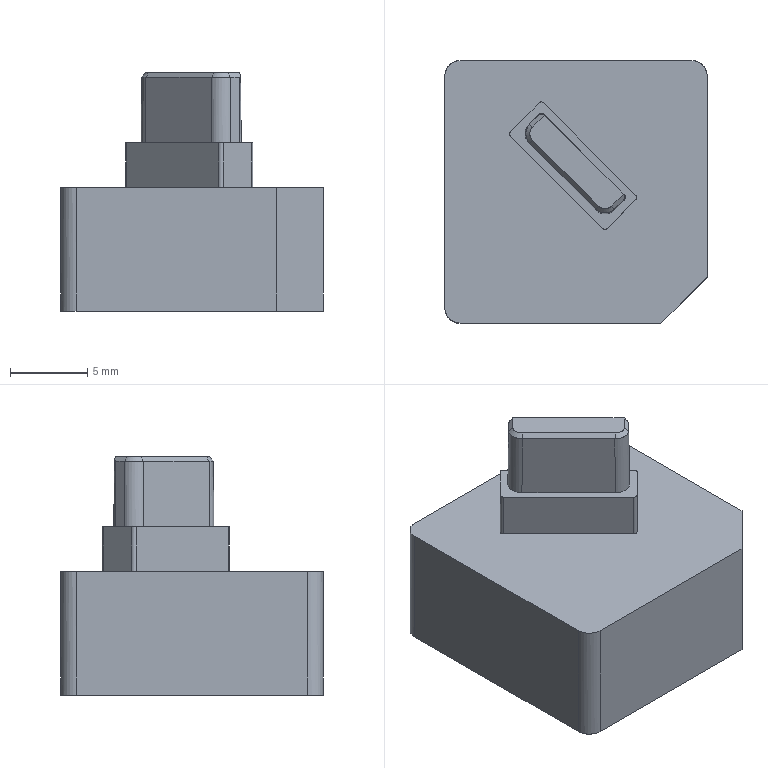NC program | PowerMill | posted with a generic post | part box 17 x 17 x 15.424 mm
Lines 38229 to 38437 of 38437:
N38326 M6
N38327 S15000 M03
N38328 G00 G90 X0.0 Y0.0
N38329 G43 Z10.304 H13
N38330
N38331 G05 P10000 R8
N38332 X-7.0355 Y-6.6806
N38333 Z-7.57
N38334 G01 Z-7.67
N38335 X-7.1957 Y-6.6713 F1000.0
N38336 X-7.3268 Y-6.6435
N38337 X-7.4288 Y-6.597
N38338 X-7.5016 Y-6.532
N38339 X-7.5453 Y-6.4484
N38340 X-7.5598 Y-6.3462
N38341 X-7.5453 Y-6.244
N38342 X-7.5016 Y-6.1604
N38343 X-7.4288 Y-6.0954
N38344 X-7.3268 Y-6.0489
N38345 X-7.1957 Y-6.0211
N38346 X-7.0355 Y-6.0118
N38347 X-6.8786 Y-6.021
N38348 X-6.7492 Y-6.0489
N38349 X-6.6473 Y-6.0953
N38350 X-6.573 Y-6.1602
N38351 X-6.5279 Y-6.2434
N38352 X-6.5128 Y-6.3462
N38353 X-6.5273 Y-6.4484
N38354 X-6.5709 Y-6.532
N38355 X-6.6435 Y-6.597
N38356 X-6.7451 Y-6.6435
N38357 X-6.8758 Y-6.6713
N38358 X-7.0355 Y-6.6806
N38359 G00 Z-4.4979
N38360 G01 X-6.5237 Y-5.0631 F10000.0
N38361 G00 Z-7.57
N38362 G01 Z-7.67 F600.0
N38363 X-7.5598 Y-5.0639 F1000.0
N38364 X-6.78 Y-5.6343
N38365 Y-4.9561
N38366 G00 Z-4.4979
N38367 G01 X-6.8918 Y-4.1114 F10000.0
N38368 G00 Z-7.57
N38369 G01 Z-7.67 F600.0
N38370 Y-4.5044 F1000.0
N38371 G00 Z-4.4979
N38372 G01 X-6.855 Y-2.7884 F10000.0
N38373 G00 Z-7.57
N38374 G01 Z-7.67 F600.0
N38375 X-6.7553 Y-2.8234 F1000.0
N38376 X-6.6717 Y-2.8732
N38377 X-6.6042 Y-2.9377
N38378 X-6.5534 Y-3.0172
N38379 X-6.523 Y-3.1089
N38380 X-6.5128 Y-3.2127
N38381 X-6.5233 Y-3.3314
N38382 X-6.5548 Y-3.4335
N38383 X-6.6073 Y-3.5192
N38384 X-6.6808 Y-3.5883
N38385 X-6.7753 Y-3.6409
N38386 X-6.9078 Y-3.6814
N38387 X-7.0504 Y-3.6948
N38388 X-7.2034 Y-3.6801
N38389 X-7.3311 Y-3.636
N38390 X-7.4335 Y-3.5625
N38391 X-7.5106 Y-3.4596
N38392 X-7.5575 Y-3.3409
N38393 X-7.5731 Y-3.2112
N38394 X-7.5646 Y-3.1148
N38395 X-7.5389 Y-3.0288
N38396 X-7.4962 Y-2.9533
N38397 X-7.4373 Y-2.89
N38398 X-7.3632 Y-2.8408
N38399 X-7.2739 Y-2.8056
N38400 G00 Z-4.4979
N38401 G01 X-7.1957 Y-2.3618 F10000.0
N38402 G00 Z-7.57
N38403 G01 Z-7.67 F600.0
N38404 X-7.3268 Y-2.334 F1000.0
N38405 X-7.4288 Y-2.2875
N38406 X-7.5016 Y-2.2225
N38407 X-7.5453 Y-2.1389
N38408 X-7.5598 Y-2.0367
N38409 X-7.5453 Y-1.9345
N38410 X-7.5016 Y-1.8509
N38411 X-7.4288 Y-1.7859
N38412 X-7.3268 Y-1.7394
N38413 X-7.1957 Y-1.7116
N38414 X-7.0355 Y-1.7023
N38415 X-6.8786 Y-1.7116
N38416 X-6.7492 Y-1.7394
N38417 X-6.6473 Y-1.7858
N38418 X-6.573 Y-1.8507
N38419 X-6.5279 Y-1.934
N38420 X-6.5128 Y-2.0367
N38421 X-6.5273 Y-2.1389
N38422 X-6.5709 Y-2.2225
N38423 X-6.6435 Y-2.2875
N38424 X-6.7451 Y-2.334
N38425 X-6.8758 Y-2.3618
N38426 X-7.0355 Y-2.3711
N38427 X-7.1957 Y-2.3618
N38428 G00 Z-4.4979
N38429 G01 X-7.4223 Y-0.9927 F10000.0
N38430 G00 Z-7.57
N38431 G01 Z-7.67 F600.0
N38432 X-7.5552 Y-0.7997 F1000.0
N38433 X-6.53
N38434 G00 Z-4.4979
N38435 G01 X-6.8918 Y0.1981 F10000.0
N38436 G00 Z-7.57
N38437 G01 Z-7.67 F600.0
N38438 Y-0.1949 F1000.0
N38439 G00 Z-4.4979
N38440 G01 X-6.5237 Y1.1225 F10000.0
N38441 G00 Z-7.57
N38442 G01 Z-7.67 F600.0
N38443 X-7.5598 Y1.1218 F1000.0
N38444 X-6.78 Y0.5514
N38445 Y1.2296
N38446 G00 Z-4.4979
N38447 G01 X-6.8918 Y2.0743 F10000.0
N38448 G00 Z-7.57
N38449 G01 Z-7.67 F600.0
N38450 Y1.6813 F1000.0
N38451 G00 Z-4.4979
N38452 G01 X-6.9385 Y2.4847 F10000.0
N38453 G00 Z-7.57
N38454 G01 Z-7.67 F600.0
N38455 X-7.0355 Y2.4791 F1000.0
N38456 X-7.1957 Y2.4884
N38457 X-7.3268 Y2.5163
N38458 X-7.4288 Y2.5627
N38459 X-7.5016 Y2.6277
N38460 X-7.5453 Y2.7113
N38461 X-7.5598 Y2.8135
N38462 X-7.5453 Y2.9157
N38463 X-7.5016 Y2.9993
N38464 X-7.4288 Y3.0643
N38465 X-7.3268 Y3.1108
N38466 X-7.1957 Y3.1387
N38467 X-7.0355 Y3.148
N38468 X-6.8786 Y3.1387
N38469 X-6.7492 Y3.1108
N38470 X-6.6473 Y3.0644
N38471 X-6.573 Y2.9995
N38472 X-6.5279 Y2.9163
N38473 X-6.5128 Y2.8135
N38474 X-6.5273 Y2.7113
N38475 X-6.5709 Y2.6277
N38476 X-6.6435 Y2.5627
N38477 X-6.7451 Y2.5163
N38478 X-6.8758 Y2.4884
N38479 X-6.9385 Y2.4847
N38480 G00 Z-4.4979
N38481 G01 X-6.5816 Y3.7106 F10000.0
N38482 G00 Z-7.57
N38483 G01 Z-7.67 F600.0
N38484 X-6.7235 F1000.0
N38485 G00 Z-4.4979
N38486 G01 X-6.8474 Y4.2917 F10000.0
N38487 G00 Z-7.57
N38488 G01 Z-7.67 F600.0
N38489 X-6.8758 Y4.2857 F1000.0
N38490 X-7.0355 Y4.2764
N38491 X-7.1957 Y4.2857
N38492 X-7.3268 Y4.3135
N38493 X-7.4288 Y4.36
N38494 X-7.5016 Y4.425
N38495 X-7.5453 Y4.5086
N38496 X-7.5598 Y4.6108
N38497 X-7.5453 Y4.713
N38498 X-7.5016 Y4.7966
N38499 X-7.4288 Y4.8616
N38500 X-7.3268 Y4.9081
N38501 X-7.1957 Y4.9359
N38502 X-7.0355 Y4.9452
N38503 X-6.8786 Y4.9359
N38504 X-6.7492 Y4.9081
N38505 X-6.6473 Y4.8617
N38506 X-6.573 Y4.7968
N38507 X-6.5279 Y4.7135
N38508 X-6.5128 Y4.6108
N38509 X-6.5273 Y4.5086
N38510 X-6.5709 Y4.425
N38511 X-6.6435 Y4.36
N38512 X-6.7451 Y4.3135
N38513 X-6.8474 Y4.2917
N38514 G00 Z-4.4979
N38515 G01 X-7.5419 Y5.3821 F10000.0
N38516 G00 Z-7.57
N38517 G01 Z-7.67 F600.0
N38518 Y6.0454 F1000.0
N38519 X-7.4557 Y6.0128
N38520 X-7.3504 Y5.9587
N38521 X-7.1668 Y5.8517
N38522 X-6.9565 Y5.7523
N38523 X-6.7442 Y5.6867
N38524 X-6.53 Y5.6548
N38525 G00 Z10.304
N38526 G05 P0
N38527 (---------------)
N38528 ( END TOOLPATH : 精公刻字01-刻字-TEXT_D4 )
N38529 (---------------)
N38530
N38531 M05
N38532 G53 Z0.0
N38533 M30
%